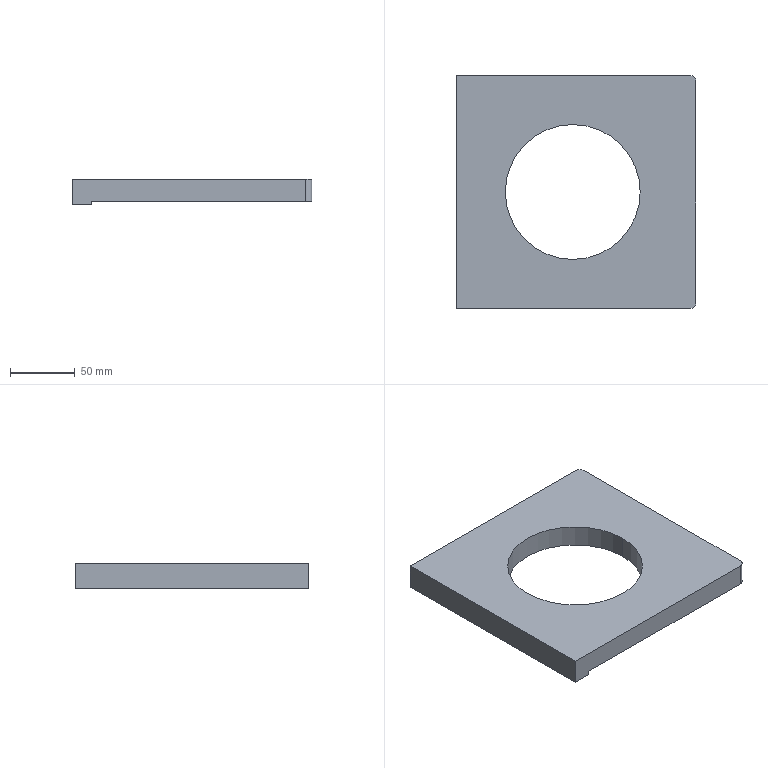Part | SolidWorks | features BaseBody 1 | 1 solid | 12 faces | box 185 x 180 x 20 mm | volume 429605 mm3 | plane 8 | cylinder 4 | commonest cylinder face diameters 10 x2 104 x2
STEP:
#1=CARTESIAN_POINT('',(-57.,0.,10.));
#2=VERTEX_POINT('',#1);
#3=CARTESIAN_POINT('',(47.,0.,10.));
#4=VERTEX_POINT('',#3);
#5=CARTESIAN_POINT('',(-5.,0.,10.));
#6=DIRECTION('',(0.,0.,1.));
#7=DIRECTION('',(1.,0.,0.));
#8=AXIS2_PLACEMENT_3D('',#5,#6,#7);
#9=CIRCLE('',#8,52.);
#10=EDGE_CURVE('',#2,#4,#9,.T.);
#11=ORIENTED_EDGE('',*,*,#10,.T.);
#12=CARTESIAN_POINT('',(47.,0.,-7.));
#13=VERTEX_POINT('',#12);
#14=CARTESIAN_POINT('',(47.,0.,10.));
#15=DIRECTION('',(0.,0.,-1.));
#16=VECTOR('',#15,1000.);
#17=LINE('',#14,#16);
#18=EDGE_CURVE('',#4,#13,#17,.T.);
#19=ORIENTED_EDGE('',*,*,#18,.T.);
#20=CARTESIAN_POINT('',(-57.,0.,-7.));
#21=VERTEX_POINT('',#20);
#22=CARTESIAN_POINT('',(-5.,0.,-7.));
#23=DIRECTION('',(0.,0.,1.));
#24=DIRECTION('',(0.,-1.,0.));
#25=AXIS2_PLACEMENT_3D('',#22,#23,#24);
#26=CIRCLE('',#25,52.);
#27=EDGE_CURVE('',#21,#13,#26,.T.);
#28=ORIENTED_EDGE('',*,*,#27,.F.);
#29=CARTESIAN_POINT('',(-57.,0.,10.));
#30=DIRECTION('',(0.,0.,-1.));
#31=VECTOR('',#30,1000.);
#32=LINE('',#29,#31);
#33=EDGE_CURVE('',#2,#21,#32,.T.);
#34=ORIENTED_EDGE('',*,*,#33,.F.);
#35=EDGE_LOOP('',(#11,#19,#28,#34));
#36=FACE_OUTER_BOUND('',#35,.T.);
#37=CARTESIAN_POINT('',(-5.,0.,10.));
#38=DIRECTION('',(0.,0.,-1.));
#39=DIRECTION('',(-1.,0.,0.));
#40=AXIS2_PLACEMENT_3D('',#37,#38,#39);
#41=CYLINDRICAL_SURFACE('',#40,52.);
#42=ADVANCED_FACE('',(#36),#41,.F.);
#43=ORIENTED_EDGE('',*,*,#10,.F.);
#44=CARTESIAN_POINT('',(-5.,0.,10.));
#45=DIRECTION('',(0.,0.,1.));
#46=DIRECTION('',(1.,0.,0.));
#47=AXIS2_PLACEMENT_3D('',#44,#45,#46);
#48=CIRCLE('',#47,52.);
#49=EDGE_CURVE('',#4,#2,#48,.T.);
#50=ORIENTED_EDGE('',*,*,#49,.F.);
#51=EDGE_LOOP('',(#43,#50));
#52=FACE_BOUND('',#51,.T.);
#53=CARTESIAN_POINT('',(90.,85.,10.));
#54=VERTEX_POINT('',#53);
#55=CARTESIAN_POINT('',(85.,90.,10.));
#56=VERTEX_POINT('',#55);
#57=CARTESIAN_POINT('',(85.,85.,10.));
#58=DIRECTION('',(0.,0.,1.));
#59=DIRECTION('',(1.,0.,0.));
#60=AXIS2_PLACEMENT_3D('',#57,#58,#59);
#61=CIRCLE('',#60,5.);
#62=EDGE_CURVE('',#54,#56,#61,.T.);
#63=ORIENTED_EDGE('',*,*,#62,.T.);
#64=CARTESIAN_POINT('',(-95.,90.,10.));
#65=VERTEX_POINT('',#64);
#66=CARTESIAN_POINT('',(0.,90.,10.));
#67=DIRECTION('',(-1.,0.,0.));
#68=VECTOR('',#67,1000.);
#69=LINE('',#66,#68);
#70=EDGE_CURVE('',#56,#65,#69,.T.);
#71=ORIENTED_EDGE('',*,*,#70,.T.);
#72=CARTESIAN_POINT('',(-95.,-90.,10.));
#73=VERTEX_POINT('',#72);
#74=CARTESIAN_POINT('',(-95.,95.,10.));
#75=DIRECTION('',(0.,-1.,0.));
#76=VECTOR('',#75,1000.);
#77=LINE('',#74,#76);
#78=EDGE_CURVE('',#65,#73,#77,.T.);
#79=ORIENTED_EDGE('',*,*,#78,.T.);
#80=CARTESIAN_POINT('',(85.,-90.,10.));
#81=VERTEX_POINT('',#80);
#82=CARTESIAN_POINT('',(0.,-90.,10.));
#83=DIRECTION('',(1.,0.,0.));
#84=VECTOR('',#83,1000.);
#85=LINE('',#82,#84);
#86=EDGE_CURVE('',#73,#81,#85,.T.);
#87=ORIENTED_EDGE('',*,*,#86,.T.);
#88=CARTESIAN_POINT('',(90.,-85.,10.));
#89=VERTEX_POINT('',#88);
#90=CARTESIAN_POINT('',(85.,-85.,10.));
#91=DIRECTION('',(0.,0.,1.));
#92=DIRECTION('',(1.,0.,0.));
#93=AXIS2_PLACEMENT_3D('',#90,#91,#92);
#94=CIRCLE('',#93,5.);
#95=EDGE_CURVE('',#81,#89,#94,.T.);
#96=ORIENTED_EDGE('',*,*,#95,.T.);
#97=CARTESIAN_POINT('',(90.,0.,10.));
#98=DIRECTION('',(0.,1.,0.));
#99=VECTOR('',#98,1000.);
#100=LINE('',#97,#99);
#101=EDGE_CURVE('',#89,#54,#100,.T.);
#102=ORIENTED_EDGE('',*,*,#101,.T.);
#103=EDGE_LOOP('',(#63,#71,#79,#87,#96,#102));
#104=FACE_OUTER_BOUND('',#103,.T.);
#105=CARTESIAN_POINT('',(0.,0.,10.));
#106=DIRECTION('',(0.,0.,1.));
#107=DIRECTION('',(1.,0.,0.));
#108=AXIS2_PLACEMENT_3D('',#105,#106,#107);
#109=PLANE('',#108);
#110=ADVANCED_FACE('',(#52,#104),#109,.T.);
#111=CARTESIAN_POINT('',(-80.,90.,-10.));
#112=VERTEX_POINT('',#111);
#113=CARTESIAN_POINT('',(-95.,90.,-10.));
#114=VERTEX_POINT('',#113);
#115=CARTESIAN_POINT('',(0.,90.,-10.));
#116=DIRECTION('',(-1.,0.,0.));
#117=VECTOR('',#116,1000.);
#118=LINE('',#115,#117);
#119=EDGE_CURVE('',#112,#114,#118,.T.);
#120=ORIENTED_EDGE('',*,*,#119,.F.);
#121=CARTESIAN_POINT('',(-80.,-90.,-10.));
#122=VERTEX_POINT('',#121);
#123=CARTESIAN_POINT('',(-80.,-95.,-10.));
#124=DIRECTION('',(0.,1.,0.));
#125=VECTOR('',#124,1000.);
#126=LINE('',#123,#125);
#127=EDGE_CURVE('',#122,#112,#126,.T.);
#128=ORIENTED_EDGE('',*,*,#127,.F.);
#129=CARTESIAN_POINT('',(-95.,-90.,-10.));
#130=VERTEX_POINT('',#129);
#131=CARTESIAN_POINT('',(0.,-90.,-10.));
#132=DIRECTION('',(1.,0.,0.));
#133=VECTOR('',#132,1000.);
#134=LINE('',#131,#133);
#135=EDGE_CURVE('',#130,#122,#134,.T.);
#136=ORIENTED_EDGE('',*,*,#135,.F.);
#137=CARTESIAN_POINT('',(-95.,95.,-10.));
#138=DIRECTION('',(0.,-1.,0.));
#139=VECTOR('',#138,1000.);
#140=LINE('',#137,#139);
#141=EDGE_CURVE('',#114,#130,#140,.T.);
#142=ORIENTED_EDGE('',*,*,#141,.F.);
#143=EDGE_LOOP('',(#120,#128,#136,#142));
#144=FACE_OUTER_BOUND('',#143,.T.);
#145=CARTESIAN_POINT('',(0.,0.,-10.));
#146=DIRECTION('',(0.,0.,1.));
#147=DIRECTION('',(1.,0.,0.));
#148=AXIS2_PLACEMENT_3D('',#145,#146,#147);
#149=PLANE('',#148);
#150=ADVANCED_FACE('',(#144),#149,.F.);
#151=CARTESIAN_POINT('',(-95.,90.,10.));
#152=DIRECTION('',(0.,0.,1.));
#153=VECTOR('',#152,1000.);
#154=LINE('',#151,#153);
#155=EDGE_CURVE('',#114,#65,#154,.T.);
#156=ORIENTED_EDGE('',*,*,#155,.F.);
#157=ORIENTED_EDGE('',*,*,#141,.T.);
#158=CARTESIAN_POINT('',(-95.,-90.,10.));
#159=DIRECTION('',(0.,0.,-1.));
#160=VECTOR('',#159,1000.);
#161=LINE('',#158,#160);
#162=EDGE_CURVE('',#73,#130,#161,.T.);
#163=ORIENTED_EDGE('',*,*,#162,.F.);
#164=ORIENTED_EDGE('',*,*,#78,.F.);
#165=EDGE_LOOP('',(#156,#157,#163,#164));
#166=FACE_OUTER_BOUND('',#165,.T.);
#167=CARTESIAN_POINT('',(-95.,95.,10.));
#168=DIRECTION('',(1.,0.,0.));
#169=DIRECTION('',(0.,0.,-1.));
#170=AXIS2_PLACEMENT_3D('',#167,#168,#169);
#171=PLANE('',#170);
#172=ADVANCED_FACE('',(#166),#171,.F.);
#173=CARTESIAN_POINT('',(-80.,90.,-7.));
#174=VERTEX_POINT('',#173);
#175=CARTESIAN_POINT('',(-80.,90.,-7.));
#176=DIRECTION('',(0.,0.,-1.));
#177=VECTOR('',#176,1000.);
#178=LINE('',#175,#177);
#179=EDGE_CURVE('',#174,#112,#178,.T.);
#180=ORIENTED_EDGE('',*,*,#179,.F.);
#181=CARTESIAN_POINT('',(-80.,-90.,-7.));
#182=VERTEX_POINT('',#181);
#183=CARTESIAN_POINT('',(-80.,-95.,-7.));
#184=DIRECTION('',(0.,1.,0.));
#185=VECTOR('',#184,1000.);
#186=LINE('',#183,#185);
#187=EDGE_CURVE('',#182,#174,#186,.T.);
#188=ORIENTED_EDGE('',*,*,#187,.F.);
#189=CARTESIAN_POINT('',(-80.,-90.,-7.));
#190=DIRECTION('',(0.,0.,1.));
#191=VECTOR('',#190,1000.);
#192=LINE('',#189,#191);
#193=EDGE_CURVE('',#122,#182,#192,.T.);
#194=ORIENTED_EDGE('',*,*,#193,.F.);
#195=ORIENTED_EDGE('',*,*,#127,.T.);
#196=EDGE_LOOP('',(#180,#188,#194,#195));
#197=FACE_OUTER_BOUND('',#196,.T.);
#198=CARTESIAN_POINT('',(-80.,-95.,-7.));
#199=DIRECTION('',(-1.,0.,0.));
#200=DIRECTION('',(0.,1.,0.));
#201=AXIS2_PLACEMENT_3D('',#198,#199,#200);
#202=PLANE('',#201);
#203=ADVANCED_FACE('',(#197),#202,.F.);
#204=ORIENTED_EDGE('',*,*,#27,.T.);
#205=CARTESIAN_POINT('',(-5.,0.,-7.));
#206=DIRECTION('',(0.,0.,1.));
#207=DIRECTION('',(0.,-1.,0.));
#208=AXIS2_PLACEMENT_3D('',#205,#206,#207);
#209=CIRCLE('',#208,52.);
#210=EDGE_CURVE('',#13,#21,#209,.T.);
#211=ORIENTED_EDGE('',*,*,#210,.T.);
#212=EDGE_LOOP('',(#204,#211));
#213=FACE_BOUND('',#212,.T.);
#214=CARTESIAN_POINT('',(85.,90.,-7.));
#215=VERTEX_POINT('',#214);
#216=CARTESIAN_POINT('',(-690.,90.,-7.));
#217=DIRECTION('',(-1.,0.,0.));
#218=VECTOR('',#217,1000.);
#219=LINE('',#216,#218);
#220=EDGE_CURVE('',#215,#174,#219,.T.);
#221=ORIENTED_EDGE('',*,*,#220,.F.);
#222=CARTESIAN_POINT('',(90.,85.,-7.));
#223=VERTEX_POINT('',#222);
#224=CARTESIAN_POINT('',(85.,85.,-7.));
#225=DIRECTION('',(0.,0.,1.));
#226=DIRECTION('',(0.,-1.,0.));
#227=AXIS2_PLACEMENT_3D('',#224,#225,#226);
#228=CIRCLE('',#227,5.);
#229=EDGE_CURVE('',#223,#215,#228,.T.);
#230=ORIENTED_EDGE('',*,*,#229,.F.);
#231=CARTESIAN_POINT('',(90.,-85.,-7.));
#232=VERTEX_POINT('',#231);
#233=CARTESIAN_POINT('',(90.,0.,-7.));
#234=DIRECTION('',(0.,1.,0.));
#235=VECTOR('',#234,1000.);
#236=LINE('',#233,#235);
#237=EDGE_CURVE('',#232,#223,#236,.T.);
#238=ORIENTED_EDGE('',*,*,#237,.F.);
#239=CARTESIAN_POINT('',(85.,-90.,-7.));
#240=VERTEX_POINT('',#239);
#241=CARTESIAN_POINT('',(85.,-85.,-7.));
#242=DIRECTION('',(0.,0.,1.));
#243=DIRECTION('',(0.,-1.,0.));
#244=AXIS2_PLACEMENT_3D('',#241,#242,#243);
#245=CIRCLE('',#244,5.);
#246=EDGE_CURVE('',#240,#232,#245,.T.);
#247=ORIENTED_EDGE('',*,*,#246,.F.);
#248=CARTESIAN_POINT('',(-690.,-90.,-7.));
#249=DIRECTION('',(1.,0.,0.));
#250=VECTOR('',#249,1000.);
#251=LINE('',#248,#250);
#252=EDGE_CURVE('',#182,#240,#251,.T.);
#253=ORIENTED_EDGE('',*,*,#252,.F.);
#254=ORIENTED_EDGE('',*,*,#187,.T.);
#255=EDGE_LOOP('',(#221,#230,#238,#247,#253,#254));
#256=FACE_OUTER_BOUND('',#255,.T.);
#257=CARTESIAN_POINT('',(-690.,0.,-7.));
#258=DIRECTION('',(0.,0.,1.));
#259=DIRECTION('',(0.,1.,0.));
#260=AXIS2_PLACEMENT_3D('',#257,#258,#259);
#261=PLANE('',#260);
#262=ADVANCED_FACE('',(#213,#256),#261,.F.);
#263=ORIENTED_EDGE('',*,*,#18,.F.);
#264=ORIENTED_EDGE('',*,*,#49,.T.);
#265=ORIENTED_EDGE('',*,*,#33,.T.);
#266=ORIENTED_EDGE('',*,*,#210,.F.);
#267=EDGE_LOOP('',(#263,#264,#265,#266));
#268=FACE_OUTER_BOUND('',#267,.T.);
#269=CARTESIAN_POINT('',(-5.,0.,10.));
#270=DIRECTION('',(0.,0.,-1.));
#271=DIRECTION('',(-1.,0.,0.));
#272=AXIS2_PLACEMENT_3D('',#269,#270,#271);
#273=CYLINDRICAL_SURFACE('',#272,52.);
#274=ADVANCED_FACE('',(#268),#273,.F.);
#275=CARTESIAN_POINT('',(90.,85.,-90.));
#276=DIRECTION('',(0.,0.,1.));
#277=VECTOR('',#276,1000.);
#278=LINE('',#275,#277);
#279=EDGE_CURVE('',#223,#54,#278,.T.);
#280=ORIENTED_EDGE('',*,*,#279,.F.);
#281=ORIENTED_EDGE('',*,*,#229,.T.);
#282=CARTESIAN_POINT('',(85.,90.,-90.));
#283=DIRECTION('',(0.,0.,1.));
#284=VECTOR('',#283,1000.);
#285=LINE('',#282,#284);
#286=EDGE_CURVE('',#215,#56,#285,.T.);
#287=ORIENTED_EDGE('',*,*,#286,.T.);
#288=ORIENTED_EDGE('',*,*,#62,.F.);
#289=EDGE_LOOP('',(#280,#281,#287,#288));
#290=FACE_OUTER_BOUND('',#289,.T.);
#291=CARTESIAN_POINT('',(85.,85.,-90.));
#292=DIRECTION('',(0.,0.,1.));
#293=DIRECTION('',(0.,1.,0.));
#294=AXIS2_PLACEMENT_3D('',#291,#292,#293);
#295=CYLINDRICAL_SURFACE('',#294,5.);
#296=ADVANCED_FACE('',(#290),#295,.T.);
#297=CARTESIAN_POINT('',(90.,-85.,-90.));
#298=DIRECTION('',(0.,0.,1.));
#299=VECTOR('',#298,1000.);
#300=LINE('',#297,#299);
#301=EDGE_CURVE('',#232,#89,#300,.T.);
#302=ORIENTED_EDGE('',*,*,#301,.F.);
#303=ORIENTED_EDGE('',*,*,#237,.T.);
#304=ORIENTED_EDGE('',*,*,#279,.T.);
#305=ORIENTED_EDGE('',*,*,#101,.F.);
#306=EDGE_LOOP('',(#302,#303,#304,#305));
#307=FACE_OUTER_BOUND('',#306,.T.);
#308=CARTESIAN_POINT('',(90.,-85.,-90.));
#309=DIRECTION('',(1.,0.,0.));
#310=DIRECTION('',(0.,-1.,0.));
#311=AXIS2_PLACEMENT_3D('',#308,#309,#310);
#312=PLANE('',#311);
#313=ADVANCED_FACE('',(#307),#312,.T.);
#314=CARTESIAN_POINT('',(85.,-90.,-90.));
#315=DIRECTION('',(0.,0.,1.));
#316=VECTOR('',#315,1000.);
#317=LINE('',#314,#316);
#318=EDGE_CURVE('',#240,#81,#317,.T.);
#319=ORIENTED_EDGE('',*,*,#318,.F.);
#320=ORIENTED_EDGE('',*,*,#246,.T.);
#321=ORIENTED_EDGE('',*,*,#301,.T.);
#322=ORIENTED_EDGE('',*,*,#95,.F.);
#323=EDGE_LOOP('',(#319,#320,#321,#322));
#324=FACE_OUTER_BOUND('',#323,.T.);
#325=CARTESIAN_POINT('',(85.,-85.,-90.));
#326=DIRECTION('',(0.,0.,1.));
#327=DIRECTION('',(0.,1.,0.));
#328=AXIS2_PLACEMENT_3D('',#325,#326,#327);
#329=CYLINDRICAL_SURFACE('',#328,5.);
#330=ADVANCED_FACE('',(#324),#329,.T.);
#331=ORIENTED_EDGE('',*,*,#286,.F.);
#332=ORIENTED_EDGE('',*,*,#220,.T.);
#333=ORIENTED_EDGE('',*,*,#179,.T.);
#334=ORIENTED_EDGE('',*,*,#119,.T.);
#335=ORIENTED_EDGE('',*,*,#155,.T.);
#336=ORIENTED_EDGE('',*,*,#70,.F.);
#337=EDGE_LOOP('',(#331,#332,#333,#334,#335,#336));
#338=FACE_OUTER_BOUND('',#337,.T.);
#339=CARTESIAN_POINT('',(85.,90.,-90.));
#340=DIRECTION('',(0.,1.,0.));
#341=DIRECTION('',(1.,0.,0.));
#342=AXIS2_PLACEMENT_3D('',#339,#340,#341);
#343=PLANE('',#342);
#344=ADVANCED_FACE('',(#338),#343,.T.);
#345=ORIENTED_EDGE('',*,*,#162,.T.);
#346=ORIENTED_EDGE('',*,*,#135,.T.);
#347=ORIENTED_EDGE('',*,*,#193,.T.);
#348=ORIENTED_EDGE('',*,*,#252,.T.);
#349=ORIENTED_EDGE('',*,*,#318,.T.);
#350=ORIENTED_EDGE('',*,*,#86,.F.);
#351=EDGE_LOOP('',(#345,#346,#347,#348,#349,#350));
#352=FACE_OUTER_BOUND('',#351,.T.);
#353=CARTESIAN_POINT('',(85.,-90.,-90.));
#354=DIRECTION('',(0.,-1.,0.));
#355=DIRECTION('',(-1.,0.,0.));
#356=AXIS2_PLACEMENT_3D('',#353,#354,#355);
#357=PLANE('',#356);
#358=ADVANCED_FACE('',(#352),#357,.T.);
#359=CLOSED_SHELL('',(#42,#110,#150,#172,#203,#262,#274,#296,#313,#330,#344,#358));
#360=MANIFOLD_SOLID_BREP('',#359);
#361=CARTESIAN_POINT('',(0.,0.,0.));
#362=DIRECTION('',(0.,0.,1.));
#363=DIRECTION('',(1.,0.,0.));
#364=AXIS2_PLACEMENT_3D('',#361,#362,#363);
#365=(LENGTH_UNIT()NAMED_UNIT(*)SI_UNIT(.MILLI.,.METRE.));
#366=UNCERTAINTY_MEASURE_WITH_UNIT(LENGTH_MEASURE(0.00001),#365,'','');
#367=(NAMED_UNIT(*)PLANE_ANGLE_UNIT()SI_UNIT($,.RADIAN.));
#368=(NAMED_UNIT(*)SI_UNIT($,.STERADIAN.)SOLID_ANGLE_UNIT());
#369=(GEOMETRIC_REPRESENTATION_CONTEXT(3)GLOBAL_UNCERTAINTY_ASSIGNED_CONTEXT((#366))GLOBAL_UNIT_ASSIGNED_CONTEXT((#365,#367,#368))REPRESENTATION_CONTEXT('',''));
#370=ADVANCED_BREP_SHAPE_REPRESENTATION('',(#360,#364),#369);